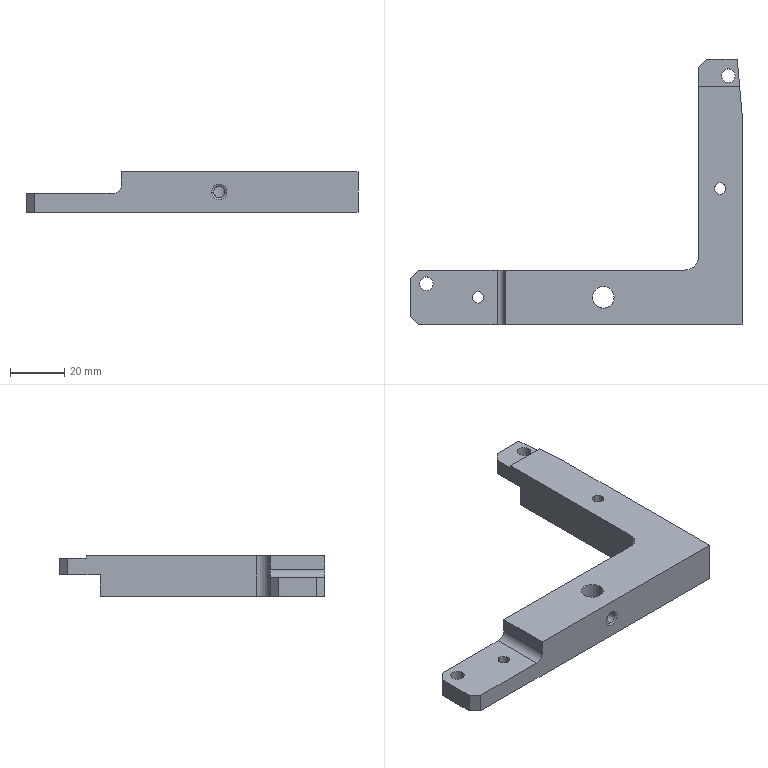Part | NX | 1 solid | 38 faces | box 122 x 97.43 x 15 mm | volume 46010 mm3 | plane 18 | cylinder 14 | cone 6 | commonest cylinder face diameters 4.2 x6 5 x4 8 x2 6 x1 10 x1
STEP:
#1=CARTESIAN_POINT('',(-29.,-10.,-115.5));
#2=VERTEX_POINT('',#1);
#3=CARTESIAN_POINT('',(-29.,10.,-115.5));
#4=VERTEX_POINT('',#3);
#5=CARTESIAN_POINT('',(-29.,-10.,-115.5));
#6=DIRECTION('',(0.,1.,0.));
#7=VECTOR('',#6,1000.);
#8=LINE('',#5,#7);
#9=EDGE_CURVE('',#2,#4,#8,.T.);
#10=ORIENTED_EDGE('',*,*,#9,.T.);
#11=CARTESIAN_POINT('',(-58.,10.,-115.5));
#12=VERTEX_POINT('',#11);
#13=CARTESIAN_POINT('',(0.,10.,-115.5));
#14=DIRECTION('',(-1.,0.,0.));
#15=VECTOR('',#14,1000.);
#16=LINE('',#13,#15);
#17=EDGE_CURVE('',#4,#12,#16,.T.);
#18=ORIENTED_EDGE('',*,*,#17,.T.);
#19=CARTESIAN_POINT('',(-61.,7.,-115.5));
#20=VERTEX_POINT('',#19);
#21=CARTESIAN_POINT('',(-68.,0.,-115.5));
#22=DIRECTION('',(-0.7071,-0.7071,0.));
#23=VECTOR('',#22,1000.);
#24=LINE('',#21,#23);
#25=EDGE_CURVE('',#12,#20,#24,.T.);
#26=ORIENTED_EDGE('',*,*,#25,.T.);
#27=CARTESIAN_POINT('',(-61.,-7.,-115.5));
#28=VERTEX_POINT('',#27);
#29=CARTESIAN_POINT('',(-61.,0.,-115.5));
#30=DIRECTION('',(0.,-1.,0.));
#31=VECTOR('',#30,1000.);
#32=LINE('',#29,#31);
#33=EDGE_CURVE('',#20,#28,#32,.T.);
#34=ORIENTED_EDGE('',*,*,#33,.T.);
#35=CARTESIAN_POINT('',(-58.,-10.,-115.5));
#36=VERTEX_POINT('',#35);
#37=CARTESIAN_POINT('',(-68.,0.,-115.5));
#38=DIRECTION('',(0.7071,-0.7071,0.));
#39=VECTOR('',#38,1000.);
#40=LINE('',#37,#39);
#41=EDGE_CURVE('',#28,#36,#40,.T.);
#42=ORIENTED_EDGE('',*,*,#41,.T.);
#43=CARTESIAN_POINT('',(0.,-10.,-115.5));
#44=DIRECTION('',(-1.,0.,0.));
#45=VECTOR('',#44,1000.);
#46=LINE('',#43,#45);
#47=EDGE_CURVE('',#2,#36,#46,.T.);
#48=ORIENTED_EDGE('',*,*,#47,.F.);
#49=EDGE_LOOP('',(#10,#18,#26,#34,#42,#48));
#50=FACE_BOUND('',#49,.T.);
#51=CARTESIAN_POINT('',(-57.5,5.,-115.5));
#52=VERTEX_POINT('',#51);
#53=CARTESIAN_POINT('',(-52.5,5.,-115.5));
#54=VERTEX_POINT('',#53);
#55=CARTESIAN_POINT('',(-55.,5.,-115.5));
#56=DIRECTION('',(0.,0.,-1.));
#57=DIRECTION('',(-1.,0.,0.));
#58=AXIS2_PLACEMENT_3D('',#55,#56,#57);
#59=CIRCLE('',#58,2.5);
#60=EDGE_CURVE('',#52,#54,#59,.T.);
#61=ORIENTED_EDGE('',*,*,#60,.T.);
#62=CARTESIAN_POINT('',(-55.,5.,-115.5));
#63=DIRECTION('',(0.,0.,-1.));
#64=DIRECTION('',(-1.,0.,0.));
#65=AXIS2_PLACEMENT_3D('',#62,#63,#64);
#66=CIRCLE('',#65,2.5);
#67=EDGE_CURVE('',#54,#52,#66,.T.);
#68=ORIENTED_EDGE('',*,*,#67,.T.);
#69=EDGE_LOOP('',(#61,#68));
#70=FACE_BOUND('',#69,.T.);
#71=CARTESIAN_POINT('',(-35.997,2.1,-115.5));
#72=VERTEX_POINT('',#71);
#73=CARTESIAN_POINT('',(-36.003,-2.1,-115.5));
#74=VERTEX_POINT('',#73);
#75=CARTESIAN_POINT('',(-36.,0.,-115.5));
#76=DIRECTION('',(0.,0.,-1.));
#77=DIRECTION('',(-0.001538,-1.,0.));
#78=AXIS2_PLACEMENT_3D('',#75,#76,#77);
#79=CIRCLE('',#78,2.1);
#80=EDGE_CURVE('',#72,#74,#79,.T.);
#81=ORIENTED_EDGE('',*,*,#80,.T.);
#82=CARTESIAN_POINT('',(-36.,0.,-115.5));
#83=DIRECTION('',(0.,0.,-1.));
#84=DIRECTION('',(-0.001538,-1.,0.));
#85=AXIS2_PLACEMENT_3D('',#82,#83,#84);
#86=CIRCLE('',#85,2.1);
#87=EDGE_CURVE('',#74,#72,#86,.T.);
#88=ORIENTED_EDGE('',*,*,#87,.T.);
#89=EDGE_LOOP('',(#81,#88));
#90=FACE_BOUND('',#89,.T.);
#91=CARTESIAN_POINT('',(-61.,10.,-115.5));
#92=DIRECTION('',(0.,0.,1.));
#93=DIRECTION('',(1.,0.,0.));
#94=AXIS2_PLACEMENT_3D('',#91,#92,#93);
#95=PLANE('',#94);
#96=ADVANCED_FACE('',(#50,#70,#90),#95,.T.);
#97=CARTESIAN_POINT('',(45.,77.63,-107.5));
#98=VERTEX_POINT('',#97);
#99=CARTESIAN_POINT('',(60.108,77.63,-107.5));
#100=VERTEX_POINT('',#99);
#101=CARTESIAN_POINT('',(0.,77.63,-107.5));
#102=DIRECTION('',(1.,0.,0.));
#103=VECTOR('',#102,1000.);
#104=LINE('',#101,#103);
#105=EDGE_CURVE('',#98,#100,#104,.T.);
#106=ORIENTED_EDGE('',*,*,#105,.T.);
#107=CARTESIAN_POINT('',(60.108,77.63,-108.5));
#108=VERTEX_POINT('',#107);
#109=CARTESIAN_POINT('',(60.108,77.63,-108.5));
#110=DIRECTION('',(0.,0.,1.));
#111=VECTOR('',#110,1000.);
#112=LINE('',#109,#111);
#113=EDGE_CURVE('',#108,#100,#112,.T.);
#114=ORIENTED_EDGE('',*,*,#113,.F.);
#115=CARTESIAN_POINT('',(45.,77.63,-108.5));
#116=VERTEX_POINT('',#115);
#117=CARTESIAN_POINT('',(45.,77.63,-108.5));
#118=DIRECTION('',(1.,0.,0.));
#119=VECTOR('',#118,1000.);
#120=LINE('',#117,#119);
#121=EDGE_CURVE('',#116,#108,#120,.T.);
#122=ORIENTED_EDGE('',*,*,#121,.F.);
#123=CARTESIAN_POINT('',(45.,77.63,-108.5));
#124=DIRECTION('',(0.,0.,1.));
#125=VECTOR('',#124,1000.);
#126=LINE('',#123,#125);
#127=EDGE_CURVE('',#116,#98,#126,.T.);
#128=ORIENTED_EDGE('',*,*,#127,.T.);
#129=EDGE_LOOP('',(#106,#114,#122,#128));
#130=FACE_BOUND('',#129,.T.);
#131=CARTESIAN_POINT('',(64.741,77.63,-107.5));
#132=DIRECTION('',(0.,1.,0.));
#133=DIRECTION('',(1.,0.,0.));
#134=AXIS2_PLACEMENT_3D('',#131,#132,#133);
#135=PLANE('',#134);
#136=ADVANCED_FACE('',(#130),#135,.T.);
#137=CARTESIAN_POINT('',(45.,84.43,-108.5));
#138=VERTEX_POINT('',#137);
#139=CARTESIAN_POINT('',(45.,77.63,-108.5));
#140=DIRECTION('',(0.,1.,0.));
#141=VECTOR('',#140,1000.);
#142=LINE('',#139,#141);
#143=EDGE_CURVE('',#116,#138,#142,.T.);
#144=ORIENTED_EDGE('',*,*,#143,.T.);
#145=CARTESIAN_POINT('',(45.,84.43,-114.5));
#146=VERTEX_POINT('',#145);
#147=CARTESIAN_POINT('',(45.,84.43,-114.5));
#148=DIRECTION('',(0.,0.,1.));
#149=VECTOR('',#148,1000.);
#150=LINE('',#147,#149);
#151=EDGE_CURVE('',#146,#138,#150,.T.);
#152=ORIENTED_EDGE('',*,*,#151,.F.);
#153=CARTESIAN_POINT('',(45.,72.43,-114.5));
#154=VERTEX_POINT('',#153);
#155=CARTESIAN_POINT('',(45.,72.43,-114.5));
#156=DIRECTION('',(0.,1.,0.));
#157=VECTOR('',#156,1000.);
#158=LINE('',#155,#157);
#159=EDGE_CURVE('',#154,#146,#158,.T.);
#160=ORIENTED_EDGE('',*,*,#159,.F.);
#161=CARTESIAN_POINT('',(45.,72.43,-122.5));
#162=VERTEX_POINT('',#161);
#163=CARTESIAN_POINT('',(45.,72.43,-114.5));
#164=DIRECTION('',(0.,0.,-1.));
#165=VECTOR('',#164,1000.);
#166=LINE('',#163,#165);
#167=EDGE_CURVE('',#154,#162,#166,.T.);
#168=ORIENTED_EDGE('',*,*,#167,.T.);
#169=CARTESIAN_POINT('',(45.,15.,-122.5));
#170=VERTEX_POINT('',#169);
#171=CARTESIAN_POINT('',(45.,0.,-122.5));
#172=DIRECTION('',(0.,-1.,0.));
#173=VECTOR('',#172,1000.);
#174=LINE('',#171,#173);
#175=EDGE_CURVE('',#162,#170,#174,.T.);
#176=ORIENTED_EDGE('',*,*,#175,.T.);
#177=CARTESIAN_POINT('',(45.,15.,-107.5));
#178=VERTEX_POINT('',#177);
#179=CARTESIAN_POINT('',(45.,15.,-122.5));
#180=DIRECTION('',(0.,0.,1.));
#181=VECTOR('',#180,1000.);
#182=LINE('',#179,#181);
#183=EDGE_CURVE('',#170,#178,#182,.T.);
#184=ORIENTED_EDGE('',*,*,#183,.T.);
#185=CARTESIAN_POINT('',(45.,0.,-107.5));
#186=DIRECTION('',(0.,-1.,0.));
#187=VECTOR('',#186,1000.);
#188=LINE('',#185,#187);
#189=EDGE_CURVE('',#98,#178,#188,.T.);
#190=ORIENTED_EDGE('',*,*,#189,.F.);
#191=ORIENTED_EDGE('',*,*,#127,.F.);
#192=EDGE_LOOP('',(#144,#152,#160,#168,#176,#184,#190,#191));
#193=FACE_BOUND('',#192,.T.);
#194=CARTESIAN_POINT('',(45.,10.,-107.5));
#195=DIRECTION('',(1.,0.,0.));
#196=DIRECTION('',(0.,1.,0.));
#197=AXIS2_PLACEMENT_3D('',#194,#195,#196);
#198=PLANE('',#197);
#199=ADVANCED_FACE('',(#193),#198,.F.);
#200=CARTESIAN_POINT('',(59.25,87.43,-108.5));
#201=VERTEX_POINT('',#200);
#202=CARTESIAN_POINT('',(48.,87.43,-108.5));
#203=VERTEX_POINT('',#202);
#204=CARTESIAN_POINT('',(59.25,87.43,-108.5));
#205=DIRECTION('',(-1.,0.,0.));
#206=VECTOR('',#205,1000.);
#207=LINE('',#204,#206);
#208=EDGE_CURVE('',#201,#203,#207,.T.);
#209=ORIENTED_EDGE('',*,*,#208,.T.);
#210=CARTESIAN_POINT('',(45.,84.43,-108.5));
#211=DIRECTION('',(0.7071,0.7071,0.));
#212=VECTOR('',#211,1000.);
#213=LINE('',#210,#212);
#214=EDGE_CURVE('',#138,#203,#213,.T.);
#215=ORIENTED_EDGE('',*,*,#214,.F.);
#216=ORIENTED_EDGE('',*,*,#143,.F.);
#217=ORIENTED_EDGE('',*,*,#121,.T.);
#218=CARTESIAN_POINT('',(59.25,87.43,-108.5));
#219=DIRECTION('',(0.08716,-0.9962,0.));
#220=VECTOR('',#219,1000.);
#221=LINE('',#218,#220);
#222=EDGE_CURVE('',#201,#108,#221,.T.);
#223=ORIENTED_EDGE('',*,*,#222,.F.);
#224=EDGE_LOOP('',(#209,#215,#216,#217,#223));
#225=FACE_BOUND('',#224,.T.);
#226=CARTESIAN_POINT('',(58.5,81.43,-108.5));
#227=VERTEX_POINT('',#226);
#228=CARTESIAN_POINT('',(53.5,81.43,-108.5));
#229=VERTEX_POINT('',#228);
#230=CARTESIAN_POINT('',(56.,81.43,-108.5));
#231=DIRECTION('',(0.,0.,1.));
#232=DIRECTION('',(-1.,0.,0.));
#233=AXIS2_PLACEMENT_3D('',#230,#231,#232);
#234=CIRCLE('',#233,2.5);
#235=EDGE_CURVE('',#227,#229,#234,.T.);
#236=ORIENTED_EDGE('',*,*,#235,.F.);
#237=CARTESIAN_POINT('',(56.,81.43,-108.5));
#238=DIRECTION('',(0.,0.,1.));
#239=DIRECTION('',(-1.,0.,0.));
#240=AXIS2_PLACEMENT_3D('',#237,#238,#239);
#241=CIRCLE('',#240,2.5);
#242=EDGE_CURVE('',#229,#227,#241,.T.);
#243=ORIENTED_EDGE('',*,*,#242,.F.);
#244=EDGE_LOOP('',(#236,#243));
#245=FACE_BOUND('',#244,.T.);
#246=CARTESIAN_POINT('',(0.,0.,-108.5));
#247=DIRECTION('',(0.,0.,-1.));
#248=DIRECTION('',(0.,-1.,0.));
#249=AXIS2_PLACEMENT_3D('',#246,#247,#248);
#250=PLANE('',#249);
#251=ADVANCED_FACE('',(#225,#245),#250,.F.);
#252=ORIENTED_EDGE('',*,*,#208,.F.);
#253=CARTESIAN_POINT('',(59.25,87.43,-114.5));
#254=VERTEX_POINT('',#253);
#255=CARTESIAN_POINT('',(59.25,87.43,-108.5));
#256=DIRECTION('',(0.,0.,-1.));
#257=VECTOR('',#256,1000.);
#258=LINE('',#255,#257);
#259=EDGE_CURVE('',#201,#254,#258,.T.);
#260=ORIENTED_EDGE('',*,*,#259,.T.);
#261=CARTESIAN_POINT('',(48.,87.43,-114.5));
#262=VERTEX_POINT('',#261);
#263=CARTESIAN_POINT('',(59.25,87.43,-114.5));
#264=DIRECTION('',(-1.,0.,0.));
#265=VECTOR('',#264,1000.);
#266=LINE('',#263,#265);
#267=EDGE_CURVE('',#254,#262,#266,.T.);
#268=ORIENTED_EDGE('',*,*,#267,.T.);
#269=CARTESIAN_POINT('',(48.,87.43,-114.5));
#270=DIRECTION('',(0.,0.,1.));
#271=VECTOR('',#270,1000.);
#272=LINE('',#269,#271);
#273=EDGE_CURVE('',#262,#203,#272,.T.);
#274=ORIENTED_EDGE('',*,*,#273,.T.);
#275=EDGE_LOOP('',(#252,#260,#268,#274));
#276=FACE_BOUND('',#275,.T.);
#277=CARTESIAN_POINT('',(0.,87.43,-107.5));
#278=DIRECTION('',(0.,-1.,0.));
#279=DIRECTION('',(0.,0.,-1.));
#280=AXIS2_PLACEMENT_3D('',#277,#278,#279);
#281=PLANE('',#280);
#282=ADVANCED_FACE('',(#276),#281,.F.);
#283=ORIENTED_EDGE('',*,*,#214,.T.);
#284=ORIENTED_EDGE('',*,*,#273,.F.);
#285=CARTESIAN_POINT('',(48.,87.43,-114.5));
#286=DIRECTION('',(-0.7071,-0.7071,0.));
#287=VECTOR('',#286,1000.);
#288=LINE('',#285,#287);
#289=EDGE_CURVE('',#262,#146,#288,.T.);
#290=ORIENTED_EDGE('',*,*,#289,.T.);
#291=ORIENTED_EDGE('',*,*,#151,.T.);
#292=EDGE_LOOP('',(#283,#284,#290,#291));
#293=FACE_BOUND('',#292,.T.);
#294=CARTESIAN_POINT('',(48.,87.43,-107.5));
#295=DIRECTION('',(-0.7071,0.7071,0.));
#296=DIRECTION('',(0.,0.,1.));
#297=AXIS2_PLACEMENT_3D('',#294,#295,#296);
#298=PLANE('',#297);
#299=ADVANCED_FACE('',(#293),#298,.T.);
#300=CARTESIAN_POINT('',(60.563,72.43,-114.5));
#301=VERTEX_POINT('',#300);
#302=CARTESIAN_POINT('',(60.563,72.43,-114.5));
#303=DIRECTION('',(-1.,0.,0.));
#304=VECTOR('',#303,1000.);
#305=LINE('',#302,#304);
#306=EDGE_CURVE('',#301,#154,#305,.T.);
#307=ORIENTED_EDGE('',*,*,#306,.T.);
#308=ORIENTED_EDGE('',*,*,#159,.T.);
#309=ORIENTED_EDGE('',*,*,#289,.F.);
#310=ORIENTED_EDGE('',*,*,#267,.F.);
#311=CARTESIAN_POINT('',(60.563,72.43,-114.5));
#312=DIRECTION('',(-0.08716,0.9962,0.));
#313=VECTOR('',#312,1000.);
#314=LINE('',#311,#313);
#315=EDGE_CURVE('',#301,#254,#314,.T.);
#316=ORIENTED_EDGE('',*,*,#315,.F.);
#317=EDGE_LOOP('',(#307,#308,#309,#310,#316));
#318=FACE_BOUND('',#317,.T.);
#319=CARTESIAN_POINT('',(53.5,81.43,-114.5));
#320=VERTEX_POINT('',#319);
#321=CARTESIAN_POINT('',(58.5,81.43,-114.5));
#322=VERTEX_POINT('',#321);
#323=CARTESIAN_POINT('',(56.,81.43,-114.5));
#324=DIRECTION('',(0.,0.,-1.));
#325=DIRECTION('',(1.,0.,0.));
#326=AXIS2_PLACEMENT_3D('',#323,#324,#325);
#327=CIRCLE('',#326,2.5);
#328=EDGE_CURVE('',#320,#322,#327,.T.);
#329=ORIENTED_EDGE('',*,*,#328,.F.);
#330=CARTESIAN_POINT('',(56.,81.43,-114.5));
#331=DIRECTION('',(0.,0.,-1.));
#332=DIRECTION('',(1.,0.,0.));
#333=AXIS2_PLACEMENT_3D('',#330,#331,#332);
#334=CIRCLE('',#333,2.5);
#335=EDGE_CURVE('',#322,#320,#334,.T.);
#336=ORIENTED_EDGE('',*,*,#335,.F.);
#337=EDGE_LOOP('',(#329,#336));
#338=FACE_BOUND('',#337,.T.);
#339=CARTESIAN_POINT('',(45.,87.43,-114.5));
#340=DIRECTION('',(0.,0.,-1.));
#341=DIRECTION('',(0.,-1.,0.));
#342=AXIS2_PLACEMENT_3D('',#339,#340,#341);
#343=PLANE('',#342);
#344=ADVANCED_FACE('',(#318,#338),#343,.T.);
#345=ORIENTED_EDGE('',*,*,#306,.F.);
#346=CARTESIAN_POINT('',(60.563,72.43,-122.5));
#347=VERTEX_POINT('',#346);
#348=CARTESIAN_POINT('',(60.563,72.43,-122.5));
#349=DIRECTION('',(0.,0.,1.));
#350=VECTOR('',#349,1000.);
#351=LINE('',#348,#350);
#352=EDGE_CURVE('',#347,#301,#351,.T.);
#353=ORIENTED_EDGE('',*,*,#352,.F.);
#354=CARTESIAN_POINT('',(0.,72.43,-122.5));
#355=DIRECTION('',(1.,0.,0.));
#356=VECTOR('',#355,1000.);
#357=LINE('',#354,#356);
#358=EDGE_CURVE('',#162,#347,#357,.T.);
#359=ORIENTED_EDGE('',*,*,#358,.F.);
#360=ORIENTED_EDGE('',*,*,#167,.F.);
#361=EDGE_LOOP('',(#345,#353,#359,#360));
#362=FACE_BOUND('',#361,.T.);
#363=CARTESIAN_POINT('',(45.,72.43,-114.5));
#364=DIRECTION('',(0.,1.,0.));
#365=DIRECTION('',(1.,0.,0.));
#366=AXIS2_PLACEMENT_3D('',#363,#364,#365);
#367=PLANE('',#366);
#368=ADVANCED_FACE('',(#362),#367,.T.);
#369=CARTESIAN_POINT('',(61.,67.43,-122.5));
#370=VERTEX_POINT('',#369);
#371=CARTESIAN_POINT('',(66.899,0.,-122.5));
#372=DIRECTION('',(0.08716,-0.9962,0.));
#373=VECTOR('',#372,1000.);
#374=LINE('',#371,#373);
#375=EDGE_CURVE('',#347,#370,#374,.T.);
#376=ORIENTED_EDGE('',*,*,#375,.T.);
#377=CARTESIAN_POINT('',(61.,-10.,-122.5));
#378=VERTEX_POINT('',#377);
#379=CARTESIAN_POINT('',(61.,0.,-122.5));
#380=DIRECTION('',(0.,1.,0.));
#381=VECTOR('',#380,1000.);
#382=LINE('',#379,#381);
#383=EDGE_CURVE('',#378,#370,#382,.T.);
#384=ORIENTED_EDGE('',*,*,#383,.F.);
#385=CARTESIAN_POINT('',(-58.,-10.,-122.5));
#386=VERTEX_POINT('',#385);
#387=CARTESIAN_POINT('',(0.,-10.,-122.5));
#388=DIRECTION('',(-1.,0.,0.));
#389=VECTOR('',#388,1000.);
#390=LINE('',#387,#389);
#391=EDGE_CURVE('',#378,#386,#390,.T.);
#392=ORIENTED_EDGE('',*,*,#391,.T.);
#393=CARTESIAN_POINT('',(-61.,-7.,-122.5));
#394=VERTEX_POINT('',#393);
#395=CARTESIAN_POINT('',(-68.,0.,-122.5));
#396=DIRECTION('',(0.7071,-0.7071,0.));
#397=VECTOR('',#396,1000.);
#398=LINE('',#395,#397);
#399=EDGE_CURVE('',#394,#386,#398,.T.);
#400=ORIENTED_EDGE('',*,*,#399,.F.);
#401=CARTESIAN_POINT('',(-61.,7.,-122.5));
#402=VERTEX_POINT('',#401);
#403=CARTESIAN_POINT('',(-61.,0.,-122.5));
#404=DIRECTION('',(0.,-1.,0.));
#405=VECTOR('',#404,1000.);
#406=LINE('',#403,#405);
#407=EDGE_CURVE('',#402,#394,#406,.T.);
#408=ORIENTED_EDGE('',*,*,#407,.F.);
#409=CARTESIAN_POINT('',(-58.,10.,-122.5));
#410=VERTEX_POINT('',#409);
#411=CARTESIAN_POINT('',(-68.,0.,-122.5));
#412=DIRECTION('',(-0.7071,-0.7071,0.));
#413=VECTOR('',#412,1000.);
#414=LINE('',#411,#413);
#415=EDGE_CURVE('',#410,#402,#414,.T.);
#416=ORIENTED_EDGE('',*,*,#415,.F.);
#417=CARTESIAN_POINT('',(40.,10.,-122.5));
#418=VERTEX_POINT('',#417);
#419=CARTESIAN_POINT('',(0.,10.,-122.5));
#420=DIRECTION('',(-1.,0.,0.));
#421=VECTOR('',#420,1000.);
#422=LINE('',#419,#421);
#423=EDGE_CURVE('',#418,#410,#422,.T.);
#424=ORIENTED_EDGE('',*,*,#423,.F.);
#425=CARTESIAN_POINT('',(40.,15.,-122.5));
#426=DIRECTION('',(0.,0.,1.));
#427=DIRECTION('',(0.,-1.,0.));
#428=AXIS2_PLACEMENT_3D('',#425,#426,#427);
#429=CIRCLE('',#428,5.);
#430=EDGE_CURVE('',#418,#170,#429,.T.);
#431=ORIENTED_EDGE('',*,*,#430,.T.);
#432=ORIENTED_EDGE('',*,*,#175,.F.);
#433=ORIENTED_EDGE('',*,*,#358,.T.);
#434=EDGE_LOOP('',(#376,#384,#392,#400,#408,#416,#424,#431,#432,#433));
#435=FACE_BOUND('',#434,.T.);
#436=CARTESIAN_POINT('',(-57.5,5.,-122.5));
#437=VERTEX_POINT('',#436);
#438=CARTESIAN_POINT('',(-52.5,5.,-122.5));
#439=VERTEX_POINT('',#438);
#440=CARTESIAN_POINT('',(-55.,5.,-122.5));
#441=DIRECTION('',(0.,0.,-1.));
#442=DIRECTION('',(-1.,0.,0.));
#443=AXIS2_PLACEMENT_3D('',#440,#441,#442);
#444=CIRCLE('',#443,2.5);
#445=EDGE_CURVE('',#437,#439,#444,.T.);
#446=ORIENTED_EDGE('',*,*,#445,.F.);
#447=CARTESIAN_POINT('',(-55.,5.,-122.5));
#448=DIRECTION('',(0.,0.,-1.));
#449=DIRECTION('',(-1.,0.,0.));
#450=AXIS2_PLACEMENT_3D('',#447,#448,#449);
#451=CIRCLE('',#450,2.5);
#452=EDGE_CURVE('',#439,#437,#451,.T.);
#453=ORIENTED_EDGE('',*,*,#452,.F.);
#454=EDGE_LOOP('',(#446,#453));
#455=FACE_BOUND('',#454,.T.);
#456=CARTESIAN_POINT('',(-38.86,0.,-122.5));
#457=VERTEX_POINT('',#456);
#458=CARTESIAN_POINT('',(-33.14,0.,-122.5));
#459=VERTEX_POINT('',#458);
#460=CARTESIAN_POINT('',(-36.,0.,-122.5));
#461=DIRECTION('',(0.,0.,-1.));
#462=DIRECTION('',(-1.,0.,0.));
#463=AXIS2_PLACEMENT_3D('',#460,#461,#462);
#464=CIRCLE('',#463,2.86);
#465=EDGE_CURVE('',#457,#459,#464,.T.);
#466=ORIENTED_EDGE('',*,*,#465,.F.);
#467=CARTESIAN_POINT('',(-36.,0.,-122.5));
#468=DIRECTION('',(0.,0.,-1.));
#469=DIRECTION('',(-1.,0.,0.));
#470=AXIS2_PLACEMENT_3D('',#467,#468,#469);
#471=CIRCLE('',#470,2.86);
#472=EDGE_CURVE('',#459,#457,#471,.T.);
#473=ORIENTED_EDGE('',*,*,#472,.F.);
#474=EDGE_LOOP('',(#466,#473));
#475=FACE_BOUND('',#474,.T.);
#476=CARTESIAN_POINT('',(14.,0.,-122.5));
#477=VERTEX_POINT('',#476);
#478=CARTESIAN_POINT('',(6.,0.,-122.5));
#479=VERTEX_POINT('',#478);
#480=CARTESIAN_POINT('',(10.,0.,-122.5));
#481=DIRECTION('',(0.,0.,-1.));
#482=DIRECTION('',(-1.,0.,0.));
#483=AXIS2_PLACEMENT_3D('',#480,#481,#482);
#484=CIRCLE('',#483,4.);
#485=EDGE_CURVE('',#477,#479,#484,.T.);
#486=ORIENTED_EDGE('',*,*,#485,.F.);
#487=CARTESIAN_POINT('',(10.,0.,-122.5));
#488=DIRECTION('',(0.,0.,-1.));
#489=DIRECTION('',(-1.,0.,0.));
#490=AXIS2_PLACEMENT_3D('',#487,#488,#489);
#491=CIRCLE('',#490,4.);
#492=EDGE_CURVE('',#479,#477,#491,.T.);
#493=ORIENTED_EDGE('',*,*,#492,.F.);
#494=EDGE_LOOP('',(#486,#493));
#495=FACE_BOUND('',#494,.T.);
#496=CARTESIAN_POINT('',(55.86,40.,-122.5));
#497=VERTEX_POINT('',#496);
#498=CARTESIAN_POINT('',(50.14,40.,-122.5));
#499=VERTEX_POINT('',#498);
#500=CARTESIAN_POINT('',(53.,40.,-122.5));
#501=DIRECTION('',(0.,0.,-1.));
#502=DIRECTION('',(-1.,0.,0.));
#503=AXIS2_PLACEMENT_3D('',#500,#501,#502);
#504=CIRCLE('',#503,2.86);
#505=EDGE_CURVE('',#497,#499,#504,.T.);
#506=ORIENTED_EDGE('',*,*,#505,.F.);
#507=CARTESIAN_POINT('',(53.,40.,-122.5));
#508=DIRECTION('',(0.,0.,-1.));
#509=DIRECTION('',(-1.,0.,0.));
#510=AXIS2_PLACEMENT_3D('',#507,#508,#509);
#511=CIRCLE('',#510,2.86);
#512=EDGE_CURVE('',#499,#497,#511,.T.);
#513=ORIENTED_EDGE('',*,*,#512,.F.);
#514=EDGE_LOOP('',(#506,#513));
#515=FACE_BOUND('',#514,.T.);
#516=CARTESIAN_POINT('',(0.,0.,-122.5));
#517=DIRECTION('',(0.,0.,1.));
#518=DIRECTION('',(1.,0.,0.));
#519=AXIS2_PLACEMENT_3D('',#516,#517,#518);
#520=PLANE('',#519);
#521=ADVANCED_FACE('',(#435,#455,#475,#495,#515),#520,.F.);
#522=ORIENTED_EDGE('',*,*,#222,.T.);
#523=ORIENTED_EDGE('',*,*,#113,.T.);
#524=CARTESIAN_POINT('',(61.,67.43,-107.5));
#525=VERTEX_POINT('',#524);
#526=CARTESIAN_POINT('',(66.899,0.,-107.5));
#527=DIRECTION('',(0.08716,-0.9962,0.));
#528=VECTOR('',#527,1000.);
#529=LINE('',#526,#528);
#530=EDGE_CURVE('',#100,#525,#529,.T.);
#531=ORIENTED_EDGE('',*,*,#530,.T.);
#532=CARTESIAN_POINT('',(61.,67.43,-122.5));
#533=DIRECTION('',(0.,0.,1.));
#534=VECTOR('',#533,1000.);
#535=LINE('',#532,#534);
#536=EDGE_CURVE('',#370,#525,#535,.T.);
#537=ORIENTED_EDGE('',*,*,#536,.F.);
#538=ORIENTED_EDGE('',*,*,#375,.F.);
#539=ORIENTED_EDGE('',*,*,#352,.T.);
#540=ORIENTED_EDGE('',*,*,#315,.T.);
#541=ORIENTED_EDGE('',*,*,#259,.F.);
#542=EDGE_LOOP('',(#522,#523,#531,#537,#538,#539,#540,#541));
#543=FACE_BOUND('',#542,.T.);
#544=CARTESIAN_POINT('',(61.,67.43,-107.5));
#545=DIRECTION('',(0.9962,0.08716,0.));
#546=DIRECTION('',(0.,0.,-1.));
#547=AXIS2_PLACEMENT_3D('',#544,#545,#546);
#548=PLANE('',#547);
#549=ADVANCED_FACE('',(#543),#548,.T.);
#550=CARTESIAN_POINT('',(61.,-10.,-107.5));
#551=VERTEX_POINT('',#550);
#552=CARTESIAN_POINT('',(61.,0.,-107.5));
#553=DIRECTION('',(0.,1.,0.));
#554=VECTOR('',#553,1000.);
#555=LINE('',#552,#554);
#556=EDGE_CURVE('',#551,#525,#555,.T.);
#557=ORIENTED_EDGE('',*,*,#556,.F.);
#558=CARTESIAN_POINT('',(61.,-10.,0.));
#559=DIRECTION('',(0.,0.,-1.));
#560=VECTOR('',#559,1000.);
#561=LINE('',#558,#560);
#562=EDGE_CURVE('',#551,#378,#561,.T.);
#563=ORIENTED_EDGE('',*,*,#562,.T.);
#564=ORIENTED_EDGE('',*,*,#383,.T.);
#565=ORIENTED_EDGE('',*,*,#536,.T.);
#566=EDGE_LOOP('',(#557,#563,#564,#565));
#567=FACE_BOUND('',#566,.T.);
#568=CARTESIAN_POINT('',(61.,-10.,-107.5));
#569=DIRECTION('',(-1.,0.,0.));
#570=DIRECTION('',(0.,0.,1.));
#571=AXIS2_PLACEMENT_3D('',#568,#569,#570);
#572=PLANE('',#571);
#573=ADVANCED_FACE('',(#567),#572,.F.);
#574=ORIENTED_EDGE('',*,*,#47,.T.);
#575=CARTESIAN_POINT('',(-58.,-10.,0.));
#576=DIRECTION('',(0.,0.,1.));
#577=VECTOR('',#576,1000.);
#578=LINE('',#575,#577);
#579=EDGE_CURVE('',#386,#36,#578,.T.);
#580=ORIENTED_EDGE('',*,*,#579,.F.);
#581=ORIENTED_EDGE('',*,*,#391,.F.);
#582=ORIENTED_EDGE('',*,*,#562,.F.);
#583=CARTESIAN_POINT('',(-26.,-10.,-107.5));
#584=VERTEX_POINT('',#583);
#585=CARTESIAN_POINT('',(0.,-10.,-107.5));
#586=DIRECTION('',(-1.,0.,0.));
#587=VECTOR('',#586,1000.);
#588=LINE('',#585,#587);
#589=EDGE_CURVE('',#551,#584,#588,.T.);
#590=ORIENTED_EDGE('',*,*,#589,.T.);
#591=CARTESIAN_POINT('',(-26.,-10.,-112.5));
#592=VERTEX_POINT('',#591);
#593=CARTESIAN_POINT('',(-26.,-10.,0.));
#594=DIRECTION('',(0.,0.,-1.));
#595=VECTOR('',#594,1000.);
#596=LINE('',#593,#595);
#597=EDGE_CURVE('',#584,#592,#596,.T.);
#598=ORIENTED_EDGE('',*,*,#597,.T.);
#599=CARTESIAN_POINT('',(-29.,-10.,-112.5));
#600=DIRECTION('',(0.,1.,0.));
#601=DIRECTION('',(1.,0.,0.));
#602=AXIS2_PLACEMENT_3D('',#599,#600,#601);
#603=CIRCLE('',#602,3.);
#604=EDGE_CURVE('',#592,#2,#603,.T.);
#605=ORIENTED_EDGE('',*,*,#604,.T.);
#606=EDGE_LOOP('',(#574,#580,#581,#582,#590,#598,#605));
#607=FACE_BOUND('',#606,.T.);
#608=CARTESIAN_POINT('',(7.14,-10.,-115.));
#609=VERTEX_POINT('',#608);
#610=CARTESIAN_POINT('',(12.86,-10.,-115.));
#611=VERTEX_POINT('',#610);
#612=CARTESIAN_POINT('',(10.,-10.,-115.));
#613=DIRECTION('',(0.,-1.,0.));
#614=DIRECTION('',(-1.,0.,0.));
#615=AXIS2_PLACEMENT_3D('',#612,#613,#614);
#616=CIRCLE('',#615,2.86);
#617=EDGE_CURVE('',#609,#611,#616,.T.);
#618=ORIENTED_EDGE('',*,*,#617,.F.);
#619=CARTESIAN_POINT('',(10.,-10.,-115.));
#620=DIRECTION('',(0.,-1.,0.));
#621=DIRECTION('',(-1.,0.,0.));
#622=AXIS2_PLACEMENT_3D('',#619,#620,#621);
#623=CIRCLE('',#622,2.86);
#624=EDGE_CURVE('',#611,#609,#623,.T.);
#625=ORIENTED_EDGE('',*,*,#624,.F.);
#626=EDGE_LOOP('',(#618,#625));
#627=FACE_BOUND('',#626,.T.);
#628=CARTESIAN_POINT('',(-61.,-10.,-107.5));
#629=DIRECTION('',(0.,1.,0.));
#630=DIRECTION('',(1.,0.,0.));
#631=AXIS2_PLACEMENT_3D('',#628,#629,#630);
#632=PLANE('',#631);
#633=ADVANCED_FACE('',(#607,#627),#632,.F.);
#634=ORIENTED_EDGE('',*,*,#105,.F.);
#635=ORIENTED_EDGE('',*,*,#189,.T.);
#636=CARTESIAN_POINT('',(40.,10.,-107.5));
#637=VERTEX_POINT('',#636);
#638=CARTESIAN_POINT('',(40.,15.,-107.5));
#639=DIRECTION('',(0.,0.,1.));
#640=DIRECTION('',(0.,-1.,0.));
#641=AXIS2_PLACEMENT_3D('',#638,#639,#640);
#642=CIRCLE('',#641,5.);
#643=EDGE_CURVE('',#637,#178,#642,.T.);
#644=ORIENTED_EDGE('',*,*,#643,.F.);
#645=CARTESIAN_POINT('',(-26.,10.,-107.5));
#646=VERTEX_POINT('',#645);
#647=CARTESIAN_POINT('',(0.,10.,-107.5));
#648=DIRECTION('',(-1.,0.,0.));
#649=VECTOR('',#648,1000.);
#650=LINE('',#647,#649);
#651=EDGE_CURVE('',#637,#646,#650,.T.);
#652=ORIENTED_EDGE('',*,*,#651,.T.);
#653=CARTESIAN_POINT('',(-26.,0.,-107.5));
#654=DIRECTION('',(0.,1.,0.));
#655=VECTOR('',#654,1000.);
#656=LINE('',#653,#655);
#657=EDGE_CURVE('',#584,#646,#656,.T.);
#658=ORIENTED_EDGE('',*,*,#657,.F.);
#659=ORIENTED_EDGE('',*,*,#589,.F.);
#660=ORIENTED_EDGE('',*,*,#556,.T.);
#661=ORIENTED_EDGE('',*,*,#530,.F.);
#662=EDGE_LOOP('',(#634,#635,#644,#652,#658,#659,#660,#661));
#663=FACE_BOUND('',#662,.T.);
#664=CARTESIAN_POINT('',(6.,0.,-107.5));
#665=VERTEX_POINT('',#664);
#666=CARTESIAN_POINT('',(14.,0.,-107.5));
#667=VERTEX_POINT('',#666);
#668=CARTESIAN_POINT('',(10.,0.,-107.5));
#669=DIRECTION('',(0.,0.,-1.));
#670=DIRECTION('',(-1.,0.,0.));
#671=AXIS2_PLACEMENT_3D('',#668,#669,#670);
#672=CIRCLE('',#671,4.);
#673=EDGE_CURVE('',#665,#667,#672,.T.);
#674=ORIENTED_EDGE('',*,*,#673,.T.);
#675=CARTESIAN_POINT('',(10.,0.,-107.5));
#676=DIRECTION('',(0.,0.,-1.));
#677=DIRECTION('',(-1.,0.,0.));
#678=AXIS2_PLACEMENT_3D('',#675,#676,#677);
#679=CIRCLE('',#678,4.);
#680=EDGE_CURVE('',#667,#665,#679,.T.);
#681=ORIENTED_EDGE('',*,*,#680,.T.);
#682=EDGE_LOOP('',(#674,#681));
#683=FACE_BOUND('',#682,.T.);
#684=CARTESIAN_POINT('',(53.003,42.1,-107.5));
#685=VERTEX_POINT('',#684);
#686=CARTESIAN_POINT('',(52.997,37.9,-107.5));
#687=VERTEX_POINT('',#686);
#688=CARTESIAN_POINT('',(53.,40.,-107.5));
#689=DIRECTION('',(0.,0.,-1.));
#690=DIRECTION('',(-0.001538,-1.,0.));
#691=AXIS2_PLACEMENT_3D('',#688,#689,#690);
#692=CIRCLE('',#691,2.1);
#693=EDGE_CURVE('',#685,#687,#692,.T.);
#694=ORIENTED_EDGE('',*,*,#693,.T.);
#695=CARTESIAN_POINT('',(53.,40.,-107.5));
#696=DIRECTION('',(0.,0.,-1.));
#697=DIRECTION('',(-0.001538,-1.,0.));
#698=AXIS2_PLACEMENT_3D('',#695,#696,#697);
#699=CIRCLE('',#698,2.1);
#700=EDGE_CURVE('',#687,#685,#699,.T.);
#701=ORIENTED_EDGE('',*,*,#700,.T.);
#702=EDGE_LOOP('',(#694,#701));
#703=FACE_BOUND('',#702,.T.);
#704=CARTESIAN_POINT('',(0.,0.,-107.5));
#705=DIRECTION('',(0.,0.,1.));
#706=DIRECTION('',(1.,0.,0.));
#707=AXIS2_PLACEMENT_3D('',#704,#705,#706);
#708=PLANE('',#707);
#709=ADVANCED_FACE('',(#663,#683,#703),#708,.T.);
#710=CARTESIAN_POINT('',(-26.,10.,-112.5));
#711=VERTEX_POINT('',#710);
#712=CARTESIAN_POINT('',(-26.,-10.272,-112.5));
#713=DIRECTION('',(0.,1.,0.));
#714=VECTOR('',#713,1000.);
#715=LINE('',#712,#714);
#716=EDGE_CURVE('',#592,#711,#715,.T.);
#717=ORIENTED_EDGE('',*,*,#716,.T.);
#718=CARTESIAN_POINT('',(-29.,10.,-112.5));
#719=DIRECTION('',(0.,1.,0.));
#720=DIRECTION('',(1.,0.,0.));
#721=AXIS2_PLACEMENT_3D('',#718,#719,#720);
#722=CIRCLE('',#721,3.);
#723=EDGE_CURVE('',#711,#4,#722,.T.);
#724=ORIENTED_EDGE('',*,*,#723,.T.);
#725=ORIENTED_EDGE('',*,*,#9,.F.);
#726=ORIENTED_EDGE('',*,*,#604,.F.);
#727=EDGE_LOOP('',(#717,#724,#725,#726));
#728=FACE_BOUND('',#727,.T.);
#729=CARTESIAN_POINT('',(-29.,-10.272,-112.5));
#730=DIRECTION('',(0.,1.,0.));
#731=DIRECTION('',(1.,0.,0.));
#732=AXIS2_PLACEMENT_3D('',#729,#730,#731);
#733=CYLINDRICAL_SURFACE('',#732,3.);
#734=ADVANCED_FACE('',(#728),#733,.F.);
#735=ORIENTED_EDGE('',*,*,#716,.F.);
#736=ORIENTED_EDGE('',*,*,#597,.F.);
#737=ORIENTED_EDGE('',*,*,#657,.T.);
#738=CARTESIAN_POINT('',(-26.,10.,-112.5));
#739=DIRECTION('',(0.,0.,1.));
#740=VECTOR('',#739,1000.);
#741=LINE('',#738,#740);
#742=EDGE_CURVE('',#711,#646,#741,.T.);
#743=ORIENTED_EDGE('',*,*,#742,.F.);
#744=EDGE_LOOP('',(#735,#736,#737,#743));
#745=FACE_BOUND('',#744,.T.);
#746=CARTESIAN_POINT('',(-26.,10.,-115.5));
#747=DIRECTION('',(-1.,0.,0.));
#748=DIRECTION('',(0.,0.,1.));
#749=AXIS2_PLACEMENT_3D('',#746,#747,#748);
#750=PLANE('',#749);
#751=ADVANCED_FACE('',(#745),#750,.T.);
#752=ORIENTED_EDGE('',*,*,#742,.T.);
#753=ORIENTED_EDGE('',*,*,#651,.F.);
#754=CARTESIAN_POINT('',(40.,10.,-107.263));
#755=DIRECTION('',(0.,0.,1.));
#756=VECTOR('',#755,1000.);
#757=LINE('',#754,#756);
#758=EDGE_CURVE('',#418,#637,#757,.T.);
#759=ORIENTED_EDGE('',*,*,#758,.F.);
#760=ORIENTED_EDGE('',*,*,#423,.T.);
#761=CARTESIAN_POINT('',(-58.,10.,-122.5));
#762=DIRECTION('',(0.,0.,1.));
#763=VECTOR('',#762,1000.);
#764=LINE('',#761,#763);
#765=EDGE_CURVE('',#410,#12,#764,.T.);
#766=ORIENTED_EDGE('',*,*,#765,.T.);
#767=ORIENTED_EDGE('',*,*,#17,.F.);
#768=ORIENTED_EDGE('',*,*,#723,.F.);
#769=EDGE_LOOP('',(#752,#753,#759,#760,#766,#767,#768));
#770=FACE_BOUND('',#769,.T.);
#771=CARTESIAN_POINT('',(61.,10.,-107.5));
#772=DIRECTION('',(0.,-1.,0.));
#773=DIRECTION('',(0.,0.,-1.));
#774=AXIS2_PLACEMENT_3D('',#771,#772,#773);
#775=PLANE('',#774);
#776=ADVANCED_FACE('',(#770),#775,.F.);
#777=CARTESIAN_POINT('',(-61.,7.,-122.5));
#778=DIRECTION('',(0.,0.,1.));
#779=VECTOR('',#778,1000.);
#780=LINE('',#777,#779);
#781=EDGE_CURVE('',#402,#20,#780,.T.);
#782=ORIENTED_EDGE('',*,*,#781,.T.);
#783=ORIENTED_EDGE('',*,*,#25,.F.);
#784=ORIENTED_EDGE('',*,*,#765,.F.);
#785=ORIENTED_EDGE('',*,*,#415,.T.);
#786=EDGE_LOOP('',(#782,#783,#784,#785));
#787=FACE_BOUND('',#786,.T.);
#788=CARTESIAN_POINT('',(-61.,7.,-107.5));
#789=DIRECTION('',(0.7071,-0.7071,0.));
#790=DIRECTION('',(0.,0.,-1.));
#791=AXIS2_PLACEMENT_3D('',#788,#789,#790);
#792=PLANE('',#791);
#793=ADVANCED_FACE('',(#787),#792,.F.);
#794=ORIENTED_EDGE('',*,*,#781,.F.);
#795=ORIENTED_EDGE('',*,*,#407,.T.);
#796=CARTESIAN_POINT('',(-61.,-7.,-122.5));
#797=DIRECTION('',(0.,0.,1.));
#798=VECTOR('',#797,1000.);
#799=LINE('',#796,#798);
#800=EDGE_CURVE('',#394,#28,#799,.T.);
#801=ORIENTED_EDGE('',*,*,#800,.T.);
#802=ORIENTED_EDGE('',*,*,#33,.F.);
#803=EDGE_LOOP('',(#794,#795,#801,#802));
#804=FACE_BOUND('',#803,.T.);
#805=CARTESIAN_POINT('',(-61.,10.,-107.5));
#806=DIRECTION('',(1.,0.,0.));
#807=DIRECTION('',(0.,1.,0.));
#808=AXIS2_PLACEMENT_3D('',#805,#806,#807);
#809=PLANE('',#808);
#810=ADVANCED_FACE('',(#804),#809,.F.);
#811=ORIENTED_EDGE('',*,*,#579,.T.);
#812=ORIENTED_EDGE('',*,*,#41,.F.);
#813=ORIENTED_EDGE('',*,*,#800,.F.);
#814=ORIENTED_EDGE('',*,*,#399,.T.);
#815=EDGE_LOOP('',(#811,#812,#813,#814));
#816=FACE_BOUND('',#815,.T.);
#817=CARTESIAN_POINT('',(-58.,-10.,-107.5));
#818=DIRECTION('',(0.7071,0.7071,0.));
#819=DIRECTION('',(0.,0.,-1.));
#820=AXIS2_PLACEMENT_3D('',#817,#818,#819);
#821=PLANE('',#820);
#822=ADVANCED_FACE('',(#816),#821,.F.);
#823=ORIENTED_EDGE('',*,*,#758,.T.);
#824=ORIENTED_EDGE('',*,*,#643,.T.);
#825=ORIENTED_EDGE('',*,*,#183,.F.);
#826=ORIENTED_EDGE('',*,*,#430,.F.);
#827=EDGE_LOOP('',(#823,#824,#825,#826));
#828=FACE_BOUND('',#827,.T.);
#829=CARTESIAN_POINT('',(40.,15.,-107.263));
#830=DIRECTION('',(0.,0.,1.));
#831=DIRECTION('',(0.,-1.,0.));
#832=AXIS2_PLACEMENT_3D('',#829,#830,#831);
#833=CYLINDRICAL_SURFACE('',#832,5.);
#834=ADVANCED_FACE('',(#828),#833,.F.);
#835=ORIENTED_EDGE('',*,*,#445,.T.);
#836=CARTESIAN_POINT('',(-52.5,5.,-122.5));
#837=DIRECTION('',(0.,0.,-1.));
#838=VECTOR('',#837,1000.);
#839=LINE('',#836,#838);
#840=EDGE_CURVE('',#439,#54,#839,.F.);
#841=ORIENTED_EDGE('',*,*,#840,.T.);
#842=ORIENTED_EDGE('',*,*,#60,.F.);
#843=CARTESIAN_POINT('',(-57.5,5.,-122.5));
#844=DIRECTION('',(0.,0.,-1.));
#845=VECTOR('',#844,1000.);
#846=LINE('',#843,#845);
#847=EDGE_CURVE('',#437,#52,#846,.F.);
#848=ORIENTED_EDGE('',*,*,#847,.F.);
#849=EDGE_LOOP('',(#835,#841,#842,#848));
#850=FACE_BOUND('',#849,.T.);
#851=CARTESIAN_POINT('',(-55.,5.,-122.5));
#852=DIRECTION('',(0.,0.,-1.));
#853=DIRECTION('',(-1.,0.,0.));
#854=AXIS2_PLACEMENT_3D('',#851,#852,#853);
#855=CYLINDRICAL_SURFACE('',#854,2.5);
#856=ADVANCED_FACE('',(#850),#855,.F.);
#857=CARTESIAN_POINT('',(-38.1,0.,-122.061));
#858=VERTEX_POINT('',#857);
#859=CARTESIAN_POINT('',(-35.997,2.1,-122.061));
#860=VERTEX_POINT('',#859);
#861=CARTESIAN_POINT('',(-36.,0.,-122.061));
#862=DIRECTION('',(0.,0.,-1.));
#863=DIRECTION('',(-1.,0.,0.));
#864=AXIS2_PLACEMENT_3D('',#861,#862,#863);
#865=CIRCLE('',#864,2.1);
#866=EDGE_CURVE('',#858,#860,#865,.T.);
#867=ORIENTED_EDGE('',*,*,#866,.F.);
#868=CARTESIAN_POINT('',(-38.86,0.,-122.5));
#869=DIRECTION('',(-0.866,0.,-0.5));
#870=VECTOR('',#869,1000.);
#871=LINE('',#868,#870);
#872=EDGE_CURVE('',#457,#858,#871,.F.);
#873=ORIENTED_EDGE('',*,*,#872,.F.);
#874=ORIENTED_EDGE('',*,*,#465,.T.);
#875=CARTESIAN_POINT('',(-33.9,0.,-122.061));
#876=VERTEX_POINT('',#875);
#877=CARTESIAN_POINT('',(-33.14,0.,-122.5));
#878=DIRECTION('',(0.866,0.,-0.5));
#879=VECTOR('',#878,1000.);
#880=LINE('',#877,#879);
#881=EDGE_CURVE('',#459,#876,#880,.F.);
#882=ORIENTED_EDGE('',*,*,#881,.T.);
#883=CARTESIAN_POINT('',(-36.,0.,-122.061));
#884=DIRECTION('',(0.,0.,-1.));
#885=DIRECTION('',(-1.,0.,0.));
#886=AXIS2_PLACEMENT_3D('',#883,#884,#885);
#887=CIRCLE('',#886,2.1);
#888=EDGE_CURVE('',#860,#876,#887,.T.);
#889=ORIENTED_EDGE('',*,*,#888,.F.);
#890=EDGE_LOOP('',(#867,#873,#874,#882,#889));
#891=FACE_BOUND('',#890,.T.);
#892=CARTESIAN_POINT('',(-36.,0.,-122.5));
#893=DIRECTION('',(0.,0.,-1.));
#894=DIRECTION('',(-1.,0.,0.));
#895=AXIS2_PLACEMENT_3D('',#892,#893,#894);
#896=CONICAL_SURFACE('',#895,2.86,1.047);
#897=ADVANCED_FACE('',(#891),#896,.F.);
#898=ORIENTED_EDGE('',*,*,#673,.F.);
#899=CARTESIAN_POINT('',(6.,0.,-122.5));
#900=DIRECTION('',(0.,0.,-1.));
#901=VECTOR('',#900,1000.);
#902=LINE('',#899,#901);
#903=EDGE_CURVE('',#479,#665,#902,.F.);
#904=ORIENTED_EDGE('',*,*,#903,.F.);
#905=ORIENTED_EDGE('',*,*,#492,.T.);
#906=CARTESIAN_POINT('',(14.,0.,-122.5));
#907=DIRECTION('',(0.,0.,-1.));
#908=VECTOR('',#907,1000.);
#909=LINE('',#906,#908);
#910=EDGE_CURVE('',#477,#667,#909,.F.);
#911=ORIENTED_EDGE('',*,*,#910,.T.);
#912=EDGE_LOOP('',(#898,#904,#905,#911));
#913=FACE_BOUND('',#912,.T.);
#914=CARTESIAN_POINT('',(10.,0.,-122.5));
#915=DIRECTION('',(0.,0.,-1.));
#916=DIRECTION('',(-1.,0.,0.));
#917=AXIS2_PLACEMENT_3D('',#914,#915,#916);
#918=CYLINDRICAL_SURFACE('',#917,4.);
#919=ADVANCED_FACE('',(#913),#918,.F.);
#920=ORIENTED_EDGE('',*,*,#328,.T.);
#921=CARTESIAN_POINT('',(58.5,81.43,-122.5));
#922=DIRECTION('',(0.,0.,-1.));
#923=VECTOR('',#922,1000.);
#924=LINE('',#921,#923);
#925=EDGE_CURVE('',#322,#227,#924,.F.);
#926=ORIENTED_EDGE('',*,*,#925,.T.);
#927=ORIENTED_EDGE('',*,*,#235,.T.);
#928=CARTESIAN_POINT('',(53.5,81.43,-122.5));
#929=DIRECTION('',(0.,0.,-1.));
#930=VECTOR('',#929,1000.);
#931=LINE('',#928,#930);
#932=EDGE_CURVE('',#320,#229,#931,.F.);
#933=ORIENTED_EDGE('',*,*,#932,.F.);
#934=EDGE_LOOP('',(#920,#926,#927,#933));
#935=FACE_BOUND('',#934,.T.);
#936=CARTESIAN_POINT('',(56.,81.43,-122.5));
#937=DIRECTION('',(0.,0.,-1.));
#938=DIRECTION('',(-1.,0.,0.));
#939=AXIS2_PLACEMENT_3D('',#936,#937,#938);
#940=CYLINDRICAL_SURFACE('',#939,2.5);
#941=ADVANCED_FACE('',(#935),#940,.F.);
#942=CARTESIAN_POINT('',(52.997,37.9,-122.061));
#943=VERTEX_POINT('',#942);
#944=CARTESIAN_POINT('',(50.9,40.,-122.061));
#945=VERTEX_POINT('',#944);
#946=CARTESIAN_POINT('',(53.,40.,-122.061));
#947=DIRECTION('',(0.,0.,-1.));
#948=DIRECTION('',(-1.,0.,0.));
#949=AXIS2_PLACEMENT_3D('',#946,#947,#948);
#950=CIRCLE('',#949,2.1);
#951=EDGE_CURVE('',#943,#945,#950,.T.);
#952=ORIENTED_EDGE('',*,*,#951,.T.);
#953=CARTESIAN_POINT('',(53.003,42.1,-122.061));
#954=VERTEX_POINT('',#953);
#955=CARTESIAN_POINT('',(53.,40.,-122.061));
#956=DIRECTION('',(0.,0.,-1.));
#957=DIRECTION('',(-1.,0.,0.));
#958=AXIS2_PLACEMENT_3D('',#955,#956,#957);
#959=CIRCLE('',#958,2.1);
#960=EDGE_CURVE('',#945,#954,#959,.T.);
#961=ORIENTED_EDGE('',*,*,#960,.T.);
#962=CARTESIAN_POINT('',(53.003,42.1,-115.));
#963=DIRECTION('',(0.,0.,-1.));
#964=VECTOR('',#963,1000.);
#965=LINE('',#962,#964);
#966=EDGE_CURVE('',#685,#954,#965,.T.);
#967=ORIENTED_EDGE('',*,*,#966,.F.);
#968=ORIENTED_EDGE('',*,*,#700,.F.);
#969=CARTESIAN_POINT('',(52.997,37.9,-115.));
#970=DIRECTION('',(0.,0.,-1.));
#971=VECTOR('',#970,1000.);
#972=LINE('',#969,#971);
#973=EDGE_CURVE('',#687,#943,#972,.T.);
#974=ORIENTED_EDGE('',*,*,#973,.T.);
#975=EDGE_LOOP('',(#952,#961,#967,#968,#974));
#976=FACE_BOUND('',#975,.T.);
#977=CARTESIAN_POINT('',(53.,40.,-115.));
#978=DIRECTION('',(0.,0.,-1.));
#979=DIRECTION('',(-0.001538,-1.,0.));
#980=AXIS2_PLACEMENT_3D('',#977,#978,#979);
#981=CYLINDRICAL_SURFACE('',#980,2.1);
#982=ADVANCED_FACE('',(#976),#981,.F.);
#983=ORIENTED_EDGE('',*,*,#951,.F.);
#984=CARTESIAN_POINT('',(55.1,40.,-122.061));
#985=VERTEX_POINT('',#984);
#986=CARTESIAN_POINT('',(53.,40.,-122.061));
#987=DIRECTION('',(0.,0.,-1.));
#988=DIRECTION('',(-1.,0.,0.));
#989=AXIS2_PLACEMENT_3D('',#986,#987,#988);
#990=CIRCLE('',#989,2.1);
#991=EDGE_CURVE('',#985,#943,#990,.T.);
#992=ORIENTED_EDGE('',*,*,#991,.F.);
#993=CARTESIAN_POINT('',(55.1,40.,-122.061));
#994=DIRECTION('',(0.866,0.,-0.5));
#995=VECTOR('',#994,1000.);
#996=LINE('',#993,#995);
#997=EDGE_CURVE('',#497,#985,#996,.F.);
#998=ORIENTED_EDGE('',*,*,#997,.F.);
#999=ORIENTED_EDGE('',*,*,#505,.T.);
#1000=CARTESIAN_POINT('',(50.9,40.,-122.061));
#1001=DIRECTION('',(-0.866,0.,-0.5));
#1002=VECTOR('',#1001,1000.);
#1003=LINE('',#1000,#1002);
#1004=EDGE_CURVE('',#499,#945,#1003,.F.);
#1005=ORIENTED_EDGE('',*,*,#1004,.T.);
#1006=EDGE_LOOP('',(#983,#992,#998,#999,#1005));
#1007=FACE_BOUND('',#1006,.T.);
#1008=CARTESIAN_POINT('',(53.,40.,-122.061));
#1009=DIRECTION('',(0.,0.,-1.));
#1010=DIRECTION('',(-1.,0.,0.));
#1011=AXIS2_PLACEMENT_3D('',#1008,#1009,#1010);
#1012=CONICAL_SURFACE('',#1011,2.1,1.047);
#1013=ADVANCED_FACE('',(#1007),#1012,.F.);
#1014=ORIENTED_EDGE('',*,*,#80,.F.);
#1015=CARTESIAN_POINT('',(-35.997,2.1,-119.));
#1016=DIRECTION('',(0.,0.,-1.));
#1017=VECTOR('',#1016,1000.);
#1018=LINE('',#1015,#1017);
#1019=EDGE_CURVE('',#72,#860,#1018,.T.);
#1020=ORIENTED_EDGE('',*,*,#1019,.T.);
#1021=ORIENTED_EDGE('',*,*,#888,.T.);
#1022=CARTESIAN_POINT('',(-36.003,-2.1,-122.061));
#1023=VERTEX_POINT('',#1022);
#1024=CARTESIAN_POINT('',(-36.,0.,-122.061));
#1025=DIRECTION('',(0.,0.,-1.));
#1026=DIRECTION('',(-1.,0.,0.));
#1027=AXIS2_PLACEMENT_3D('',#1024,#1025,#1026);
#1028=CIRCLE('',#1027,2.1);
#1029=EDGE_CURVE('',#876,#1023,#1028,.T.);
#1030=ORIENTED_EDGE('',*,*,#1029,.T.);
#1031=CARTESIAN_POINT('',(-36.003,-2.1,-119.));
#1032=DIRECTION('',(0.,0.,-1.));
#1033=VECTOR('',#1032,1000.);
#1034=LINE('',#1031,#1033);
#1035=EDGE_CURVE('',#74,#1023,#1034,.T.);
#1036=ORIENTED_EDGE('',*,*,#1035,.F.);
#1037=EDGE_LOOP('',(#1014,#1020,#1021,#1030,#1036));
#1038=FACE_BOUND('',#1037,.T.);
#1039=CARTESIAN_POINT('',(-36.,0.,-119.));
#1040=DIRECTION('',(0.,0.,-1.));
#1041=DIRECTION('',(-0.001538,-1.,0.));
#1042=AXIS2_PLACEMENT_3D('',#1039,#1040,#1041);
#1043=CYLINDRICAL_SURFACE('',#1042,2.1);
#1044=ADVANCED_FACE('',(#1038),#1043,.F.);
#1045=CARTESIAN_POINT('',(10.,-9.561,-117.1));
#1046=VERTEX_POINT('',#1045);
#1047=CARTESIAN_POINT('',(12.1,-9.561,-115.));
#1048=VERTEX_POINT('',#1047);
#1049=CARTESIAN_POINT('',(10.,-9.561,-115.));
#1050=DIRECTION('',(0.,-1.,0.));
#1051=DIRECTION('',(-1.,0.,0.));
#1052=AXIS2_PLACEMENT_3D('',#1049,#1050,#1051);
#1053=CIRCLE('',#1052,2.1);
#1054=EDGE_CURVE('',#1046,#1048,#1053,.T.);
#1055=ORIENTED_EDGE('',*,*,#1054,.T.);
#1056=CARTESIAN_POINT('',(10.,-9.561,-112.9));
#1057=VERTEX_POINT('',#1056);
#1058=CARTESIAN_POINT('',(10.,-9.561,-115.));
#1059=DIRECTION('',(0.,-1.,0.));
#1060=DIRECTION('',(-1.,0.,0.));
#1061=AXIS2_PLACEMENT_3D('',#1058,#1059,#1060);
#1062=CIRCLE('',#1061,2.1);
#1063=EDGE_CURVE('',#1048,#1057,#1062,.T.);
#1064=ORIENTED_EDGE('',*,*,#1063,.T.);
#1065=CARTESIAN_POINT('',(10.,-4.,-112.9));
#1066=VERTEX_POINT('',#1065);
#1067=CARTESIAN_POINT('',(10.,-6.702,-112.9));
#1068=DIRECTION('',(0.,-1.,0.));
#1069=VECTOR('',#1068,1000.);
#1070=LINE('',#1067,#1069);
#1071=EDGE_CURVE('',#1066,#1057,#1070,.T.);
#1072=ORIENTED_EDGE('',*,*,#1071,.F.);
#1073=CARTESIAN_POINT('',(10.,-4.,-117.1));
#1074=VERTEX_POINT('',#1073);
#1075=CARTESIAN_POINT('',(10.,-4.,-112.9));
#1076=CARTESIAN_POINT('',(10.266,-4.,-112.9));
#1077=CARTESIAN_POINT('',(10.74,-3.944,-113.006));
#1078=CARTESIAN_POINT('',(11.117,-3.843,-113.214));
#1079=CARTESIAN_POINT('',(11.414,-3.748,-113.421));
#1080=CARTESIAN_POINT('',(11.692,-3.626,-113.75));
#1081=CARTESIAN_POINT('',(11.73,-3.607,-113.806));
#1082=CARTESIAN_POINT('',(11.866,-3.539,-114.027));
#1083=CARTESIAN_POINT('',(11.96,-3.487,-114.231));
#1084=CARTESIAN_POINT('',(12.081,-3.418,-114.612));
#1085=CARTESIAN_POINT('',(12.109,-3.398,-115.));
#1086=CARTESIAN_POINT('',(12.081,-3.418,-115.389));
#1087=CARTESIAN_POINT('',(11.96,-3.487,-115.77));
#1088=CARTESIAN_POINT('',(11.865,-3.539,-115.974));
#1089=CARTESIAN_POINT('',(11.729,-3.607,-116.195));
#1090=CARTESIAN_POINT('',(11.692,-3.626,-116.249));
#1091=CARTESIAN_POINT('',(11.412,-3.748,-116.581));
#1092=CARTESIAN_POINT('',(11.116,-3.843,-116.786));
#1093=CARTESIAN_POINT('',(10.74,-3.944,-116.994));
#1094=CARTESIAN_POINT('',(10.266,-4.,-117.1));
#1095=CARTESIAN_POINT('',(10.,-4.,-117.1));
#1096=B_SPLINE_CURVE_WITH_KNOTS('',3,(#1075,#1076,#1077,#1078,#1079,#1080,#1081,#1082,#1083,#1084,#1085,#1086,#1087,#1088,#1089,#1090,#1091,#1092,#1093,#1094,#1095),.UNSPECIFIED.,.F.,.F.,(4,1,1,1,1,1,1,1,1,1,1,1,1,1,1,1,1,1,4),(0.,0.125,0.1875,0.25,0.2812,0.3125,0.3438,0.375,0.4375,0.5,0.5625,0.625,0.6562,0.6875,0.7188,0.75,0.8125,0.875,1.),.UNSPECIFIED.);
#1097=EDGE_CURVE('',#1074,#1066,#1096,.F.);
#1098=ORIENTED_EDGE('',*,*,#1097,.F.);
#1099=CARTESIAN_POINT('',(10.,-6.702,-117.1));
#1100=DIRECTION('',(0.,-1.,0.));
#1101=VECTOR('',#1100,1000.);
#1102=LINE('',#1099,#1101);
#1103=EDGE_CURVE('',#1074,#1046,#1102,.T.);
#1104=ORIENTED_EDGE('',*,*,#1103,.T.);
#1105=EDGE_LOOP('',(#1055,#1064,#1072,#1098,#1104));
#1106=FACE_BOUND('',#1105,.T.);
#1107=CARTESIAN_POINT('',(10.,-6.702,-115.));
#1108=DIRECTION('',(0.,-1.,0.));
#1109=DIRECTION('',(0.,0.,1.));
#1110=AXIS2_PLACEMENT_3D('',#1107,#1108,#1109);
#1111=CYLINDRICAL_SURFACE('',#1110,2.1);
#1112=ADVANCED_FACE('',(#1106),#1111,.F.);
#1113=ORIENTED_EDGE('',*,*,#617,.T.);
#1114=CARTESIAN_POINT('',(12.1,-9.561,-115.));
#1115=DIRECTION('',(0.866,-0.5,0.));
#1116=VECTOR('',#1115,1000.);
#1117=LINE('',#1114,#1116);
#1118=EDGE_CURVE('',#1048,#611,#1117,.T.);
#1119=ORIENTED_EDGE('',*,*,#1118,.F.);
#1120=ORIENTED_EDGE('',*,*,#1054,.F.);
#1121=CARTESIAN_POINT('',(7.9,-9.561,-115.));
#1122=VERTEX_POINT('',#1121);
#1123=CARTESIAN_POINT('',(10.,-9.561,-115.));
#1124=DIRECTION('',(0.,-1.,0.));
#1125=DIRECTION('',(-1.,0.,0.));
#1126=AXIS2_PLACEMENT_3D('',#1123,#1124,#1125);
#1127=CIRCLE('',#1126,2.1);
#1128=EDGE_CURVE('',#1122,#1046,#1127,.T.);
#1129=ORIENTED_EDGE('',*,*,#1128,.F.);
#1130=CARTESIAN_POINT('',(7.9,-9.561,-115.));
#1131=DIRECTION('',(-0.866,-0.5,0.));
#1132=VECTOR('',#1131,1000.);
#1133=LINE('',#1130,#1132);
#1134=EDGE_CURVE('',#1122,#609,#1133,.T.);
#1135=ORIENTED_EDGE('',*,*,#1134,.T.);
#1136=EDGE_LOOP('',(#1113,#1119,#1120,#1129,#1135));
#1137=FACE_BOUND('',#1136,.T.);
#1138=CARTESIAN_POINT('',(10.,-9.561,-115.));
#1139=DIRECTION('',(0.,-1.,0.));
#1140=DIRECTION('',(-1.,0.,0.));
#1141=AXIS2_PLACEMENT_3D('',#1138,#1139,#1140);
#1142=CONICAL_SURFACE('',#1141,2.1,1.047);
#1143=ADVANCED_FACE('',(#1137),#1142,.F.);
#1144=ORIENTED_EDGE('',*,*,#932,.T.);
#1145=ORIENTED_EDGE('',*,*,#242,.T.);
#1146=ORIENTED_EDGE('',*,*,#925,.F.);
#1147=ORIENTED_EDGE('',*,*,#335,.T.);
#1148=EDGE_LOOP('',(#1144,#1145,#1146,#1147));
#1149=FACE_BOUND('',#1148,.T.);
#1150=CARTESIAN_POINT('',(56.,81.43,-122.5));
#1151=DIRECTION('',(0.,0.,-1.));
#1152=DIRECTION('',(-1.,0.,0.));
#1153=AXIS2_PLACEMENT_3D('',#1150,#1151,#1152);
#1154=CYLINDRICAL_SURFACE('',#1153,2.5);
#1155=ADVANCED_FACE('',(#1149),#1154,.F.);
#1156=ORIENTED_EDGE('',*,*,#872,.T.);
#1157=CARTESIAN_POINT('',(-36.,0.,-122.061));
#1158=DIRECTION('',(0.,0.,-1.));
#1159=DIRECTION('',(-1.,0.,0.));
#1160=AXIS2_PLACEMENT_3D('',#1157,#1158,#1159);
#1161=CIRCLE('',#1160,2.1);
#1162=EDGE_CURVE('',#1023,#858,#1161,.T.);
#1163=ORIENTED_EDGE('',*,*,#1162,.F.);
#1164=ORIENTED_EDGE('',*,*,#1029,.F.);
#1165=ORIENTED_EDGE('',*,*,#881,.F.);
#1166=ORIENTED_EDGE('',*,*,#472,.T.);
#1167=EDGE_LOOP('',(#1156,#1163,#1164,#1165,#1166));
#1168=FACE_BOUND('',#1167,.T.);
#1169=CARTESIAN_POINT('',(-36.,0.,-122.5));
#1170=DIRECTION('',(0.,0.,-1.));
#1171=DIRECTION('',(-1.,0.,0.));
#1172=AXIS2_PLACEMENT_3D('',#1169,#1170,#1171);
#1173=CONICAL_SURFACE('',#1172,2.86,1.047);
#1174=ADVANCED_FACE('',(#1168),#1173,.F.);
#1175=ORIENTED_EDGE('',*,*,#1118,.T.);
#1176=ORIENTED_EDGE('',*,*,#624,.T.);
#1177=ORIENTED_EDGE('',*,*,#1134,.F.);
#1178=CARTESIAN_POINT('',(10.,-9.561,-115.));
#1179=DIRECTION('',(0.,-1.,0.));
#1180=DIRECTION('',(-1.,0.,0.));
#1181=AXIS2_PLACEMENT_3D('',#1178,#1179,#1180);
#1182=CIRCLE('',#1181,2.1);
#1183=EDGE_CURVE('',#1057,#1122,#1182,.T.);
#1184=ORIENTED_EDGE('',*,*,#1183,.F.);
#1185=ORIENTED_EDGE('',*,*,#1063,.F.);
#1186=EDGE_LOOP('',(#1175,#1176,#1177,#1184,#1185));
#1187=FACE_BOUND('',#1186,.T.);
#1188=CARTESIAN_POINT('',(10.,-9.561,-115.));
#1189=DIRECTION('',(0.,-1.,0.));
#1190=DIRECTION('',(-1.,0.,0.));
#1191=AXIS2_PLACEMENT_3D('',#1188,#1189,#1190);
#1192=CONICAL_SURFACE('',#1191,2.1,1.047);
#1193=ADVANCED_FACE('',(#1187),#1192,.F.);
#1194=ORIENTED_EDGE('',*,*,#693,.F.);
#1195=ORIENTED_EDGE('',*,*,#966,.T.);
#1196=CARTESIAN_POINT('',(53.,40.,-122.061));
#1197=DIRECTION('',(0.,0.,-1.));
#1198=DIRECTION('',(-1.,0.,0.));
#1199=AXIS2_PLACEMENT_3D('',#1196,#1197,#1198);
#1200=CIRCLE('',#1199,2.1);
#1201=EDGE_CURVE('',#954,#985,#1200,.T.);
#1202=ORIENTED_EDGE('',*,*,#1201,.T.);
#1203=ORIENTED_EDGE('',*,*,#991,.T.);
#1204=ORIENTED_EDGE('',*,*,#973,.F.);
#1205=EDGE_LOOP('',(#1194,#1195,#1202,#1203,#1204));
#1206=FACE_BOUND('',#1205,.T.);
#1207=CARTESIAN_POINT('',(53.,40.,-115.));
#1208=DIRECTION('',(0.,0.,-1.));
#1209=DIRECTION('',(-0.001538,-1.,0.));
#1210=AXIS2_PLACEMENT_3D('',#1207,#1208,#1209);
#1211=CYLINDRICAL_SURFACE('',#1210,2.1);
#1212=ADVANCED_FACE('',(#1206),#1211,.F.);
#1213=ORIENTED_EDGE('',*,*,#866,.T.);
#1214=ORIENTED_EDGE('',*,*,#1019,.F.);
#1215=ORIENTED_EDGE('',*,*,#87,.F.);
#1216=ORIENTED_EDGE('',*,*,#1035,.T.);
#1217=ORIENTED_EDGE('',*,*,#1162,.T.);
#1218=EDGE_LOOP('',(#1213,#1214,#1215,#1216,#1217));
#1219=FACE_BOUND('',#1218,.T.);
#1220=CARTESIAN_POINT('',(-36.,0.,-119.));
#1221=DIRECTION('',(0.,0.,-1.));
#1222=DIRECTION('',(-0.001538,-1.,0.));
#1223=AXIS2_PLACEMENT_3D('',#1220,#1221,#1222);
#1224=CYLINDRICAL_SURFACE('',#1223,2.1);
#1225=ADVANCED_FACE('',(#1219),#1224,.F.);
#1226=ORIENTED_EDGE('',*,*,#1004,.F.);
#1227=ORIENTED_EDGE('',*,*,#512,.T.);
#1228=ORIENTED_EDGE('',*,*,#997,.T.);
#1229=ORIENTED_EDGE('',*,*,#1201,.F.);
#1230=ORIENTED_EDGE('',*,*,#960,.F.);
#1231=EDGE_LOOP('',(#1226,#1227,#1228,#1229,#1230));
#1232=FACE_BOUND('',#1231,.T.);
#1233=CARTESIAN_POINT('',(53.,40.,-122.061));
#1234=DIRECTION('',(0.,0.,-1.));
#1235=DIRECTION('',(-1.,0.,0.));
#1236=AXIS2_PLACEMENT_3D('',#1233,#1234,#1235);
#1237=CONICAL_SURFACE('',#1236,2.1,1.047);
#1238=ADVANCED_FACE('',(#1232),#1237,.F.);
#1239=ORIENTED_EDGE('',*,*,#485,.T.);
#1240=ORIENTED_EDGE('',*,*,#903,.T.);
#1241=ORIENTED_EDGE('',*,*,#680,.F.);
#1242=ORIENTED_EDGE('',*,*,#910,.F.);
#1243=EDGE_LOOP('',(#1239,#1240,#1241,#1242));
#1244=FACE_BOUND('',#1243,.T.);
#1245=CARTESIAN_POINT('',(7.9,-3.404,-115.));
#1246=VERTEX_POINT('',#1245);
#1247=CARTESIAN_POINT('',(10.,-4.,-112.9));
#1248=CARTESIAN_POINT('',(8.878,-4.,-112.9));
#1249=CARTESIAN_POINT('',(7.901,-3.405,-113.886));
#1250=CARTESIAN_POINT('',(7.9,-3.404,-115.));
#1251=B_SPLINE_CURVE_WITH_KNOTS('',3,(#1247,#1248,#1249,#1250),.UNSPECIFIED.,.F.,.F.,(4,4),(0.,1.),.UNSPECIFIED.);
#1252=EDGE_CURVE('',#1066,#1246,#1251,.T.);
#1253=ORIENTED_EDGE('',*,*,#1252,.T.);
#1254=CARTESIAN_POINT('',(7.9,-3.404,-115.));
#1255=CARTESIAN_POINT('',(7.901,-3.405,-116.114));
#1256=CARTESIAN_POINT('',(8.878,-4.,-117.1));
#1257=CARTESIAN_POINT('',(10.,-4.,-117.1));
#1258=B_SPLINE_CURVE_WITH_KNOTS('',3,(#1254,#1255,#1256,#1257),.UNSPECIFIED.,.F.,.F.,(4,4),(0.,1.),.UNSPECIFIED.);
#1259=EDGE_CURVE('',#1246,#1074,#1258,.T.);
#1260=ORIENTED_EDGE('',*,*,#1259,.T.);
#1261=ORIENTED_EDGE('',*,*,#1097,.T.);
#1262=EDGE_LOOP('',(#1253,#1260,#1261));
#1263=FACE_BOUND('',#1262,.T.);
#1264=CARTESIAN_POINT('',(10.,0.,-122.5));
#1265=DIRECTION('',(0.,0.,-1.));
#1266=DIRECTION('',(-1.,0.,0.));
#1267=AXIS2_PLACEMENT_3D('',#1264,#1265,#1266);
#1268=CYLINDRICAL_SURFACE('',#1267,4.);
#1269=ADVANCED_FACE('',(#1244,#1263),#1268,.F.);
#1270=ORIENTED_EDGE('',*,*,#847,.T.);
#1271=ORIENTED_EDGE('',*,*,#67,.F.);
#1272=ORIENTED_EDGE('',*,*,#840,.F.);
#1273=ORIENTED_EDGE('',*,*,#452,.T.);
#1274=EDGE_LOOP('',(#1270,#1271,#1272,#1273));
#1275=FACE_BOUND('',#1274,.T.);
#1276=CARTESIAN_POINT('',(-55.,5.,-122.5));
#1277=DIRECTION('',(0.,0.,-1.));
#1278=DIRECTION('',(-1.,0.,0.));
#1279=AXIS2_PLACEMENT_3D('',#1276,#1277,#1278);
#1280=CYLINDRICAL_SURFACE('',#1279,2.5);
#1281=ADVANCED_FACE('',(#1275),#1280,.F.);
#1282=ORIENTED_EDGE('',*,*,#1259,.F.);
#1283=ORIENTED_EDGE('',*,*,#1252,.F.);
#1284=ORIENTED_EDGE('',*,*,#1071,.T.);
#1285=ORIENTED_EDGE('',*,*,#1183,.T.);
#1286=ORIENTED_EDGE('',*,*,#1128,.T.);
#1287=ORIENTED_EDGE('',*,*,#1103,.F.);
#1288=EDGE_LOOP('',(#1282,#1283,#1284,#1285,#1286,#1287));
#1289=FACE_BOUND('',#1288,.T.);
#1290=CARTESIAN_POINT('',(10.,-6.702,-115.));
#1291=DIRECTION('',(0.,-1.,0.));
#1292=DIRECTION('',(0.,0.,1.));
#1293=AXIS2_PLACEMENT_3D('',#1290,#1291,#1292);
#1294=CYLINDRICAL_SURFACE('',#1293,2.1);
#1295=ADVANCED_FACE('',(#1289),#1294,.F.);
#1296=CLOSED_SHELL('',(#96,#136,#199,#251,#282,#299,#344,#368,#521,#549,#573,#633,#709,#734,#751,#776,#793,#810,#822,#834,#856,#897,#919,#941,#982,#1013,#1044,#1112,#1143,#1155,#1174,#1193,#1212,#1225,#1238,#1269,#1281,#1295));
#1297=MANIFOLD_SOLID_BREP('',#1296);
#1298=(LENGTH_UNIT()NAMED_UNIT(*)SI_UNIT(.MILLI.,.METRE.));
#1299=UNCERTAINTY_MEASURE_WITH_UNIT(LENGTH_MEASURE(0.0508),#1298,'','');
#1300=(NAMED_UNIT(*)PLANE_ANGLE_UNIT()SI_UNIT($,.RADIAN.));
#1301=(NAMED_UNIT(*)SI_UNIT($,.STERADIAN.)SOLID_ANGLE_UNIT());
#1302=(GEOMETRIC_REPRESENTATION_CONTEXT(3)GLOBAL_UNCERTAINTY_ASSIGNED_CONTEXT((#1299))GLOBAL_UNIT_ASSIGNED_CONTEXT((#1298,#1300,#1301))REPRESENTATION_CONTEXT('',''));
#1303=ADVANCED_BREP_SHAPE_REPRESENTATION('',(#1297),#1302);